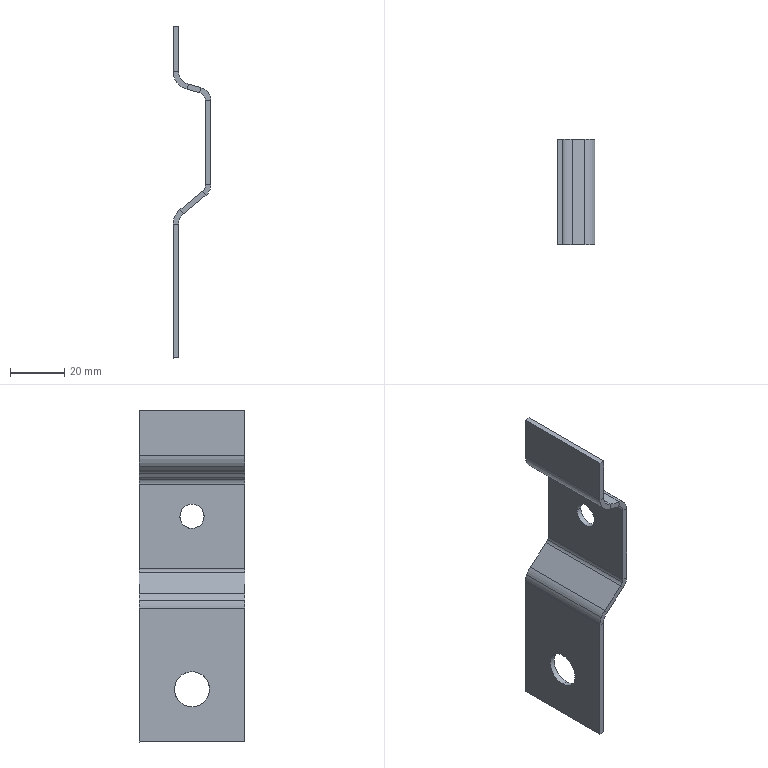Part | NX | features BREP 1 | 1 solid | 46 faces | box 14 x 39 x 122.887 mm | volume 10128 mm3 | plane 30 | cylinder 16 | commonest cylinder face diameters 6 x4 10 x4 14 x4 9 x2 13 x2
STEP:
#1=CARTESIAN_POINT('',(580.388,46.572,344.883));
#2=VERTEX_POINT('',#1);
#3=CARTESIAN_POINT('',(580.388,7.572,344.883));
#4=VERTEX_POINT('',#3);
#5=CARTESIAN_POINT('',(580.388,27.072,344.883));
#6=DIRECTION('',(0.,-1.,0.));
#7=VECTOR('',#6,1000.);
#8=LINE('',#5,#7);
#9=EDGE_CURVE('',#2,#4,#8,.T.);
#10=ORIENTED_EDGE('',*,*,#9,.F.);
#11=CARTESIAN_POINT('',(580.388,46.572,328.184));
#12=VERTEX_POINT('',#11);
#13=CARTESIAN_POINT('',(580.388,46.572,336.534));
#14=DIRECTION('',(0.,0.,1.));
#15=VECTOR('',#14,1000.);
#16=LINE('',#13,#15);
#17=EDGE_CURVE('',#12,#2,#16,.T.);
#18=ORIENTED_EDGE('',*,*,#17,.F.);
#19=CARTESIAN_POINT('',(580.388,7.572,328.184));
#20=VERTEX_POINT('',#19);
#21=CARTESIAN_POINT('',(580.388,27.072,328.184));
#22=DIRECTION('',(0.,1.,-0.000000573));
#23=VECTOR('',#22,1000.);
#24=LINE('',#21,#23);
#25=EDGE_CURVE('',#20,#12,#24,.T.);
#26=ORIENTED_EDGE('',*,*,#25,.F.);
#27=CARTESIAN_POINT('',(580.388,7.572,336.534));
#28=DIRECTION('',(0.,0.,1.));
#29=VECTOR('',#28,1000.);
#30=LINE('',#27,#29);
#31=EDGE_CURVE('',#20,#4,#30,.T.);
#32=ORIENTED_EDGE('',*,*,#31,.T.);
#33=EDGE_LOOP('',(#10,#18,#26,#32));
#34=FACE_BOUND('',#33,.T.);
#35=CARTESIAN_POINT('',(580.388,46.572,328.184));
#36=DIRECTION('',(-1.,0.,0.));
#37=DIRECTION('',(0.,-1.,0.));
#38=AXIS2_PLACEMENT_3D('',#35,#36,#37);
#39=PLANE('',#38);
#40=ADVANCED_FACE('',(#34),#39,.T.);
#41=CARTESIAN_POINT('',(582.388,46.572,344.883));
#42=VERTEX_POINT('',#41);
#43=CARTESIAN_POINT('',(581.388,46.572,344.883));
#44=DIRECTION('',(-1.,0.,0.));
#45=VECTOR('',#44,1000.);
#46=LINE('',#43,#45);
#47=EDGE_CURVE('',#42,#2,#46,.T.);
#48=ORIENTED_EDGE('',*,*,#47,.T.);
#49=ORIENTED_EDGE('',*,*,#9,.T.);
#50=CARTESIAN_POINT('',(582.388,7.572,344.883));
#51=VERTEX_POINT('',#50);
#52=CARTESIAN_POINT('',(581.388,7.572,344.883));
#53=DIRECTION('',(-1.,0.,0.));
#54=VECTOR('',#53,1000.);
#55=LINE('',#52,#54);
#56=EDGE_CURVE('',#51,#4,#55,.T.);
#57=ORIENTED_EDGE('',*,*,#56,.F.);
#58=CARTESIAN_POINT('',(582.388,27.072,344.883));
#59=DIRECTION('',(0.,-1.,0.));
#60=VECTOR('',#59,1000.);
#61=LINE('',#58,#60);
#62=EDGE_CURVE('',#42,#51,#61,.T.);
#63=ORIENTED_EDGE('',*,*,#62,.F.);
#64=EDGE_LOOP('',(#48,#49,#57,#63));
#65=FACE_BOUND('',#64,.T.);
#66=CARTESIAN_POINT('',(582.388,46.572,344.883));
#67=DIRECTION('',(0.,0.,-1.));
#68=DIRECTION('',(0.,-1.,0.));
#69=AXIS2_PLACEMENT_3D('',#66,#67,#68);
#70=PLANE('',#69);
#71=ADVANCED_FACE('',(#65),#70,.F.);
#72=CARTESIAN_POINT('',(582.388,46.572,328.184));
#73=VERTEX_POINT('',#72);
#74=CARTESIAN_POINT('',(582.388,46.572,336.534));
#75=DIRECTION('',(0.,0.,1.));
#76=VECTOR('',#75,1000.);
#77=LINE('',#74,#76);
#78=EDGE_CURVE('',#73,#42,#77,.T.);
#79=ORIENTED_EDGE('',*,*,#78,.F.);
#80=CARTESIAN_POINT('',(581.388,46.572,328.184));
#81=DIRECTION('',(-1.,0.,0.000000001));
#82=VECTOR('',#81,1000.);
#83=LINE('',#80,#82);
#84=EDGE_CURVE('',#73,#12,#83,.T.);
#85=ORIENTED_EDGE('',*,*,#84,.T.);
#86=ORIENTED_EDGE('',*,*,#17,.T.);
#87=ORIENTED_EDGE('',*,*,#47,.F.);
#88=EDGE_LOOP('',(#79,#85,#86,#87));
#89=FACE_BOUND('',#88,.T.);
#90=CARTESIAN_POINT('',(582.388,46.572,328.184));
#91=DIRECTION('',(0.,-1.,0.));
#92=DIRECTION('',(0.,0.,1.));
#93=AXIS2_PLACEMENT_3D('',#90,#91,#92);
#94=PLANE('',#93);
#95=ADVANCED_FACE('',(#89),#94,.F.);
#96=CARTESIAN_POINT('',(581.835,7.572,323.923));
#97=VERTEX_POINT('',#96);
#98=CARTESIAN_POINT('',(581.835,46.572,323.923));
#99=VERTEX_POINT('',#98);
#100=CARTESIAN_POINT('',(581.835,27.072,323.923));
#101=DIRECTION('',(0.,1.,-0.000000573));
#102=VECTOR('',#101,1000.);
#103=LINE('',#100,#102);
#104=EDGE_CURVE('',#97,#99,#103,.T.);
#105=ORIENTED_EDGE('',*,*,#104,.T.);
#106=CARTESIAN_POINT('',(585.577,46.572,321.423));
#107=VERTEX_POINT('',#106);
#108=CARTESIAN_POINT('',(587.388,46.572,328.184));
#109=DIRECTION('',(0.,1.,-0.000000573));
#110=DIRECTION('',(1.,0.,0.));
#111=AXIS2_PLACEMENT_3D('',#108,#109,#110);
#112=CIRCLE('',#111,7.);
#113=EDGE_CURVE('',#107,#99,#112,.T.);
#114=ORIENTED_EDGE('',*,*,#113,.F.);
#115=CARTESIAN_POINT('',(585.577,7.572,321.423));
#116=VERTEX_POINT('',#115);
#117=CARTESIAN_POINT('',(585.577,46.572,321.423));
#118=CARTESIAN_POINT('',(585.577,36.822,321.423));
#119=CARTESIAN_POINT('',(585.577,27.072,321.423));
#120=CARTESIAN_POINT('',(585.577,17.322,321.423));
#121=CARTESIAN_POINT('',(585.577,7.572,321.423));
#122=B_SPLINE_CURVE_WITH_KNOTS('',4,(#117,#118,#119,#120,#121),.UNSPECIFIED.,.F.,.F.,(5,5),(16.4,55.4),.UNSPECIFIED.);
#123=EDGE_CURVE('',#107,#116,#122,.T.);
#124=ORIENTED_EDGE('',*,*,#123,.T.);
#125=CARTESIAN_POINT('',(587.388,7.572,328.184));
#126=DIRECTION('',(0.,1.,-0.000000573));
#127=DIRECTION('',(1.,0.,0.));
#128=AXIS2_PLACEMENT_3D('',#125,#126,#127);
#129=CIRCLE('',#128,7.);
#130=EDGE_CURVE('',#116,#97,#129,.T.);
#131=ORIENTED_EDGE('',*,*,#130,.T.);
#132=EDGE_LOOP('',(#105,#114,#124,#131));
#133=FACE_BOUND('',#132,.T.);
#134=CARTESIAN_POINT('',(587.388,27.072,328.184));
#135=DIRECTION('',(0.,1.,-0.000000573));
#136=DIRECTION('',(0.7934,0.000000348,0.6088));
#137=AXIS2_PLACEMENT_3D('',#134,#135,#136);
#138=CYLINDRICAL_SURFACE('',#137,7.);
#139=ADVANCED_FACE('',(#133),#138,.T.);
#140=ORIENTED_EDGE('',*,*,#104,.F.);
#141=CARTESIAN_POINT('',(587.388,7.572,328.184));
#142=DIRECTION('',(0.,1.,-0.000000573));
#143=DIRECTION('',(1.,0.,0.));
#144=AXIS2_PLACEMENT_3D('',#141,#142,#143);
#145=CIRCLE('',#144,7.);
#146=EDGE_CURVE('',#97,#20,#145,.T.);
#147=ORIENTED_EDGE('',*,*,#146,.T.);
#148=ORIENTED_EDGE('',*,*,#25,.T.);
#149=CARTESIAN_POINT('',(587.388,46.572,328.184));
#150=DIRECTION('',(0.,1.,-0.000000573));
#151=DIRECTION('',(1.,0.,0.));
#152=AXIS2_PLACEMENT_3D('',#149,#150,#151);
#153=CIRCLE('',#152,7.);
#154=EDGE_CURVE('',#99,#12,#153,.T.);
#155=ORIENTED_EDGE('',*,*,#154,.F.);
#156=EDGE_LOOP('',(#140,#147,#148,#155));
#157=FACE_BOUND('',#156,.T.);
#158=CARTESIAN_POINT('',(587.388,27.072,328.184));
#159=DIRECTION('',(0.,1.,-0.000000573));
#160=DIRECTION('',(-0.7934,-0.000000348,-0.6088));
#161=AXIS2_PLACEMENT_3D('',#158,#159,#160);
#162=CYLINDRICAL_SURFACE('',#161,7.);
#163=ADVANCED_FACE('',(#157),#162,.T.);
#164=ORIENTED_EDGE('',*,*,#56,.T.);
#165=ORIENTED_EDGE('',*,*,#31,.F.);
#166=CARTESIAN_POINT('',(582.388,7.572,328.184));
#167=VERTEX_POINT('',#166);
#168=CARTESIAN_POINT('',(581.388,7.572,328.184));
#169=DIRECTION('',(-1.,0.,0.));
#170=VECTOR('',#169,1000.);
#171=LINE('',#168,#170);
#172=EDGE_CURVE('',#167,#20,#171,.T.);
#173=ORIENTED_EDGE('',*,*,#172,.F.);
#174=CARTESIAN_POINT('',(582.388,7.572,336.534));
#175=DIRECTION('',(0.,0.,1.));
#176=VECTOR('',#175,1000.);
#177=LINE('',#174,#176);
#178=EDGE_CURVE('',#167,#51,#177,.T.);
#179=ORIENTED_EDGE('',*,*,#178,.T.);
#180=EDGE_LOOP('',(#164,#165,#173,#179));
#181=FACE_BOUND('',#180,.T.);
#182=CARTESIAN_POINT('',(582.388,7.572,328.184));
#183=DIRECTION('',(0.,-1.,0.));
#184=DIRECTION('',(0.,0.,1.));
#185=AXIS2_PLACEMENT_3D('',#182,#183,#184);
#186=PLANE('',#185);
#187=ADVANCED_FACE('',(#181),#186,.T.);
#188=ORIENTED_EDGE('',*,*,#178,.F.);
#189=CARTESIAN_POINT('',(582.388,27.072,328.184));
#190=DIRECTION('',(0.,1.,-0.000000573));
#191=VECTOR('',#190,1000.);
#192=LINE('',#189,#191);
#193=EDGE_CURVE('',#167,#73,#192,.T.);
#194=ORIENTED_EDGE('',*,*,#193,.T.);
#195=ORIENTED_EDGE('',*,*,#78,.T.);
#196=ORIENTED_EDGE('',*,*,#62,.T.);
#197=EDGE_LOOP('',(#188,#194,#195,#196));
#198=FACE_BOUND('',#197,.T.);
#199=CARTESIAN_POINT('',(582.388,46.572,328.184));
#200=DIRECTION('',(-1.,0.,0.));
#201=DIRECTION('',(0.,-1.,0.));
#202=AXIS2_PLACEMENT_3D('',#199,#200,#201);
#203=PLANE('',#202);
#204=ADVANCED_FACE('',(#198),#203,.F.);
#205=CARTESIAN_POINT('',(586.094,46.572,323.355));
#206=VERTEX_POINT('',#205);
#207=CARTESIAN_POINT('',(587.388,46.572,328.184));
#208=DIRECTION('',(0.,1.,-0.000000573));
#209=DIRECTION('',(1.,0.,0.));
#210=AXIS2_PLACEMENT_3D('',#207,#208,#209);
#211=CIRCLE('',#210,5.);
#212=EDGE_CURVE('',#206,#73,#211,.T.);
#213=ORIENTED_EDGE('',*,*,#212,.F.);
#214=CARTESIAN_POINT('',(585.577,46.572,321.423));
#215=CARTESIAN_POINT('',(586.094,46.572,323.355));
#216=B_SPLINE_CURVE_WITH_KNOTS('',1,(#214,#215),.UNSPECIFIED.,.F.,.F.,(2,2),(-2.,0.),.UNSPECIFIED.);
#217=EDGE_CURVE('',#107,#206,#216,.T.);
#218=ORIENTED_EDGE('',*,*,#217,.F.);
#219=ORIENTED_EDGE('',*,*,#113,.T.);
#220=ORIENTED_EDGE('',*,*,#154,.T.);
#221=ORIENTED_EDGE('',*,*,#84,.F.);
#222=EDGE_LOOP('',(#213,#218,#219,#220,#221));
#223=FACE_BOUND('',#222,.T.);
#224=CARTESIAN_POINT('',(583.744,46.572,325.388));
#225=DIRECTION('',(0.,1.,-0.000000573));
#226=DIRECTION('',(0.7934,0.000000348,0.6088));
#227=AXIS2_PLACEMENT_3D('',#224,#225,#226);
#228=PLANE('',#227);
#229=ADVANCED_FACE('',(#223),#228,.T.);
#230=CARTESIAN_POINT('',(590.165,7.572,320.193));
#231=VERTEX_POINT('',#230);
#232=CARTESIAN_POINT('',(587.871,7.572,320.808));
#233=DIRECTION('',(0.9659,0.,-0.2588));
#234=VECTOR('',#233,1000.);
#235=LINE('',#232,#234);
#236=EDGE_CURVE('',#116,#231,#235,.T.);
#237=ORIENTED_EDGE('',*,*,#236,.F.);
#238=ORIENTED_EDGE('',*,*,#123,.F.);
#239=CARTESIAN_POINT('',(590.165,46.572,320.193));
#240=VERTEX_POINT('',#239);
#241=CARTESIAN_POINT('',(585.577,46.572,321.423));
#242=CARTESIAN_POINT('',(586.494,46.572,321.177));
#243=CARTESIAN_POINT('',(587.412,46.572,320.931));
#244=CARTESIAN_POINT('',(588.33,46.572,320.685));
#245=CARTESIAN_POINT('',(589.247,46.572,320.439));
#246=CARTESIAN_POINT('',(590.165,46.572,320.193));
#247=B_SPLINE_CURVE_WITH_KNOTS('',5,(#241,#242,#243,#244,#245,#246),.UNSPECIFIED.,.F.,.F.,(6,6),(0.,4.75),.UNSPECIFIED.);
#248=EDGE_CURVE('',#107,#240,#247,.T.);
#249=ORIENTED_EDGE('',*,*,#248,.T.);
#250=CARTESIAN_POINT('',(590.165,27.072,320.193));
#251=DIRECTION('',(0.,1.,-0.000000573));
#252=VECTOR('',#251,1000.);
#253=LINE('',#250,#252);
#254=EDGE_CURVE('',#231,#240,#253,.T.);
#255=ORIENTED_EDGE('',*,*,#254,.F.);
#256=EDGE_LOOP('',(#237,#238,#249,#255));
#257=FACE_BOUND('',#256,.T.);
#258=CARTESIAN_POINT('',(587.871,27.072,320.808));
#259=DIRECTION('',(0.2588,0.000000553,0.9659));
#260=DIRECTION('',(0.9659,0.,-0.2588));
#261=AXIS2_PLACEMENT_3D('',#258,#259,#260);
#262=PLANE('',#261);
#263=ADVANCED_FACE('',(#257),#262,.F.);
#264=ORIENTED_EDGE('',*,*,#172,.T.);
#265=ORIENTED_EDGE('',*,*,#146,.F.);
#266=ORIENTED_EDGE('',*,*,#130,.F.);
#267=CARTESIAN_POINT('',(586.094,7.572,323.355));
#268=VERTEX_POINT('',#267);
#269=CARTESIAN_POINT('',(585.835,7.572,322.389));
#270=DIRECTION('',(-0.2588,-0.000000553,-0.9659));
#271=VECTOR('',#270,1000.);
#272=LINE('',#269,#271);
#273=EDGE_CURVE('',#268,#116,#272,.T.);
#274=ORIENTED_EDGE('',*,*,#273,.F.);
#275=CARTESIAN_POINT('',(587.388,7.572,328.184));
#276=DIRECTION('',(0.,1.,-0.000000573));
#277=DIRECTION('',(1.,0.,0.));
#278=AXIS2_PLACEMENT_3D('',#275,#276,#277);
#279=CIRCLE('',#278,5.);
#280=EDGE_CURVE('',#268,#167,#279,.T.);
#281=ORIENTED_EDGE('',*,*,#280,.T.);
#282=EDGE_LOOP('',(#264,#265,#266,#274,#281));
#283=FACE_BOUND('',#282,.T.);
#284=CARTESIAN_POINT('',(583.744,7.572,325.388));
#285=DIRECTION('',(0.,1.,-0.000000573));
#286=DIRECTION('',(0.7934,0.000000348,0.6088));
#287=AXIS2_PLACEMENT_3D('',#284,#285,#286);
#288=PLANE('',#287);
#289=ADVANCED_FACE('',(#283),#288,.F.);
#290=ORIENTED_EDGE('',*,*,#280,.F.);
#291=CARTESIAN_POINT('',(586.094,46.572,323.355));
#292=CARTESIAN_POINT('',(586.094,40.472,323.355));
#293=CARTESIAN_POINT('',(586.094,34.372,323.355));
#294=CARTESIAN_POINT('',(586.094,28.272,323.355));
#295=CARTESIAN_POINT('',(586.094,20.472,323.355));
#296=CARTESIAN_POINT('',(586.094,12.672,323.355));
#297=CARTESIAN_POINT('',(586.094,10.972,323.355));
#298=CARTESIAN_POINT('',(586.094,9.272,323.355));
#299=CARTESIAN_POINT('',(586.094,7.572,323.355));
#300=B_SPLINE_CURVE_WITH_KNOTS('',5,(#291,#292,#293,#294,#295,#296,#297,#298,#299),.UNSPECIFIED.,.F.,.F.,(6,3,6),(16.4,46.9,55.4),.UNSPECIFIED.);
#301=EDGE_CURVE('',#206,#268,#300,.T.);
#302=ORIENTED_EDGE('',*,*,#301,.F.);
#303=ORIENTED_EDGE('',*,*,#212,.T.);
#304=ORIENTED_EDGE('',*,*,#193,.F.);
#305=EDGE_LOOP('',(#290,#302,#303,#304));
#306=FACE_BOUND('',#305,.T.);
#307=CARTESIAN_POINT('',(587.388,27.072,328.184));
#308=DIRECTION('',(0.,1.,-0.000000573));
#309=DIRECTION('',(-0.2588,-0.000000553,-0.9659));
#310=AXIS2_PLACEMENT_3D('',#307,#308,#309);
#311=CYLINDRICAL_SURFACE('',#310,5.);
#312=ADVANCED_FACE('',(#306),#311,.F.);
#313=CARTESIAN_POINT('',(590.683,46.572,322.125));
#314=VERTEX_POINT('',#313);
#315=CARTESIAN_POINT('',(590.424,46.572,321.159));
#316=DIRECTION('',(0.2588,0.000000553,0.9659));
#317=VECTOR('',#316,1000.);
#318=LINE('',#315,#317);
#319=EDGE_CURVE('',#240,#314,#318,.T.);
#320=ORIENTED_EDGE('',*,*,#319,.F.);
#321=ORIENTED_EDGE('',*,*,#248,.F.);
#322=ORIENTED_EDGE('',*,*,#217,.T.);
#323=CARTESIAN_POINT('',(586.094,46.572,323.355));
#324=CARTESIAN_POINT('',(587.012,46.572,323.109));
#325=CARTESIAN_POINT('',(587.93,46.572,322.863));
#326=CARTESIAN_POINT('',(588.847,46.572,322.617));
#327=CARTESIAN_POINT('',(589.765,46.572,322.371));
#328=CARTESIAN_POINT('',(590.683,46.572,322.125));
#329=B_SPLINE_CURVE_WITH_KNOTS('',5,(#323,#324,#325,#326,#327,#328),.UNSPECIFIED.,.F.,.F.,(6,6),(49.413,54.163),.UNSPECIFIED.);
#330=EDGE_CURVE('',#206,#314,#329,.T.);
#331=ORIENTED_EDGE('',*,*,#330,.T.);
#332=EDGE_LOOP('',(#320,#321,#322,#331));
#333=FACE_BOUND('',#332,.T.);
#334=CARTESIAN_POINT('',(588.13,46.572,321.774));
#335=DIRECTION('',(0.000000143,-1.,0.000000534));
#336=DIRECTION('',(0.,-0.000000534,-1.));
#337=AXIS2_PLACEMENT_3D('',#334,#335,#336);
#338=PLANE('',#337);
#339=ADVANCED_FACE('',(#333),#338,.F.);
#340=CARTESIAN_POINT('',(591.769,46.572,319.122));
#341=VERTEX_POINT('',#340);
#342=CARTESIAN_POINT('',(592.389,46.572,317.296));
#343=VERTEX_POINT('',#342);
#344=CARTESIAN_POINT('',(589.389,46.572,317.295));
#345=DIRECTION('',(0.,1.,-0.000000573));
#346=DIRECTION('',(1.,0.,0.));
#347=AXIS2_PLACEMENT_3D('',#344,#345,#346);
#348=CIRCLE('',#347,3.);
#349=EDGE_CURVE('',#341,#343,#348,.T.);
#350=ORIENTED_EDGE('',*,*,#349,.T.);
#351=CARTESIAN_POINT('',(592.389,7.572,317.296));
#352=VERTEX_POINT('',#351);
#353=CARTESIAN_POINT('',(592.389,27.072,317.296));
#354=DIRECTION('',(0.,1.,0.));
#355=VECTOR('',#354,1000.);
#356=LINE('',#353,#355);
#357=EDGE_CURVE('',#352,#343,#356,.T.);
#358=ORIENTED_EDGE('',*,*,#357,.F.);
#359=CARTESIAN_POINT('',(591.769,7.572,319.122));
#360=VERTEX_POINT('',#359);
#361=CARTESIAN_POINT('',(589.389,7.572,317.296));
#362=DIRECTION('',(0.,1.,-0.000000573));
#363=DIRECTION('',(1.,0.,0.));
#364=AXIS2_PLACEMENT_3D('',#361,#362,#363);
#365=CIRCLE('',#364,3.);
#366=EDGE_CURVE('',#360,#352,#365,.T.);
#367=ORIENTED_EDGE('',*,*,#366,.F.);
#368=CARTESIAN_POINT('',(591.769,27.072,319.122));
#369=DIRECTION('',(0.,1.,-0.000000573));
#370=VECTOR('',#369,1000.);
#371=LINE('',#368,#370);
#372=EDGE_CURVE('',#360,#341,#371,.T.);
#373=ORIENTED_EDGE('',*,*,#372,.T.);
#374=EDGE_LOOP('',(#350,#358,#367,#373));
#375=FACE_BOUND('',#374,.T.);
#376=CARTESIAN_POINT('',(589.389,27.072,317.295));
#377=DIRECTION('',(0.,1.,-0.000000573));
#378=DIRECTION('',(0.7934,0.000000348,0.6088));
#379=AXIS2_PLACEMENT_3D('',#376,#377,#378);
#380=CYLINDRICAL_SURFACE('',#379,3.);
#381=ADVANCED_FACE('',(#375),#380,.F.);
#382=CARTESIAN_POINT('',(589.389,7.572,317.296));
#383=DIRECTION('',(0.,1.,-0.000000573));
#384=DIRECTION('',(1.,0.,0.));
#385=AXIS2_PLACEMENT_3D('',#382,#383,#384);
#386=CIRCLE('',#385,3.);
#387=EDGE_CURVE('',#231,#360,#386,.T.);
#388=ORIENTED_EDGE('',*,*,#387,.F.);
#389=ORIENTED_EDGE('',*,*,#254,.T.);
#390=CARTESIAN_POINT('',(589.389,46.572,317.295));
#391=DIRECTION('',(0.,1.,-0.000000573));
#392=DIRECTION('',(1.,0.,0.));
#393=AXIS2_PLACEMENT_3D('',#390,#391,#392);
#394=CIRCLE('',#393,3.);
#395=EDGE_CURVE('',#240,#341,#394,.T.);
#396=ORIENTED_EDGE('',*,*,#395,.T.);
#397=ORIENTED_EDGE('',*,*,#372,.F.);
#398=EDGE_LOOP('',(#388,#389,#396,#397));
#399=FACE_BOUND('',#398,.T.);
#400=CARTESIAN_POINT('',(589.389,27.072,317.295));
#401=DIRECTION('',(0.,1.,-0.000000573));
#402=DIRECTION('',(-0.7934,-0.000000348,-0.6088));
#403=AXIS2_PLACEMENT_3D('',#400,#401,#402);
#404=CYLINDRICAL_SURFACE('',#403,3.);
#405=ADVANCED_FACE('',(#399),#404,.F.);
#406=CARTESIAN_POINT('',(590.683,7.572,322.125));
#407=VERTEX_POINT('',#406);
#408=CARTESIAN_POINT('',(586.094,7.572,323.355));
#409=CARTESIAN_POINT('',(587.012,7.572,323.109));
#410=CARTESIAN_POINT('',(587.93,7.572,322.863));
#411=CARTESIAN_POINT('',(588.847,7.572,322.617));
#412=CARTESIAN_POINT('',(589.765,7.572,322.371));
#413=CARTESIAN_POINT('',(590.683,7.572,322.125));
#414=B_SPLINE_CURVE_WITH_KNOTS('',5,(#408,#409,#410,#411,#412,#413),.UNSPECIFIED.,.F.,.F.,(6,6),(49.413,54.163),.UNSPECIFIED.);
#415=EDGE_CURVE('',#268,#407,#414,.T.);
#416=ORIENTED_EDGE('',*,*,#415,.F.);
#417=ORIENTED_EDGE('',*,*,#273,.T.);
#418=ORIENTED_EDGE('',*,*,#236,.T.);
#419=CARTESIAN_POINT('',(590.424,7.572,321.159));
#420=DIRECTION('',(0.2588,0.000000553,0.9659));
#421=VECTOR('',#420,1000.);
#422=LINE('',#419,#421);
#423=EDGE_CURVE('',#231,#407,#422,.T.);
#424=ORIENTED_EDGE('',*,*,#423,.T.);
#425=EDGE_LOOP('',(#416,#417,#418,#424));
#426=FACE_BOUND('',#425,.T.);
#427=CARTESIAN_POINT('',(586.094,7.572,323.355));
#428=DIRECTION('',(0.000000143,-1.,0.000000534));
#429=DIRECTION('',(0.9659,0.,-0.2588));
#430=AXIS2_PLACEMENT_3D('',#427,#428,#429);
#431=PLANE('',#430);
#432=ADVANCED_FACE('',(#426),#431,.T.);
#433=CARTESIAN_POINT('',(590.683,27.072,322.125));
#434=DIRECTION('',(0.,1.,-0.000000573));
#435=VECTOR('',#434,1000.);
#436=LINE('',#433,#435);
#437=EDGE_CURVE('',#407,#314,#436,.T.);
#438=ORIENTED_EDGE('',*,*,#437,.T.);
#439=ORIENTED_EDGE('',*,*,#330,.F.);
#440=ORIENTED_EDGE('',*,*,#301,.T.);
#441=ORIENTED_EDGE('',*,*,#415,.T.);
#442=EDGE_LOOP('',(#438,#439,#440,#441));
#443=FACE_BOUND('',#442,.T.);
#444=CARTESIAN_POINT('',(566.377,27.797,328.638));
#445=DIRECTION('',(0.2588,0.000000553,0.9659));
#446=DIRECTION('',(0.9659,0.,-0.2588));
#447=AXIS2_PLACEMENT_3D('',#444,#445,#446);
#448=PLANE('',#447);
#449=ADVANCED_FACE('',(#443),#448,.T.);
#450=CARTESIAN_POINT('',(594.389,46.572,317.295));
#451=VERTEX_POINT('',#450);
#452=CARTESIAN_POINT('',(593.389,46.572,317.295));
#453=DIRECTION('',(-1.,0.,0.));
#454=VECTOR('',#453,1000.);
#455=LINE('',#452,#454);
#456=EDGE_CURVE('',#451,#343,#455,.T.);
#457=ORIENTED_EDGE('',*,*,#456,.T.);
#458=ORIENTED_EDGE('',*,*,#349,.F.);
#459=ORIENTED_EDGE('',*,*,#395,.F.);
#460=ORIENTED_EDGE('',*,*,#319,.T.);
#461=CARTESIAN_POINT('',(589.389,46.572,317.295));
#462=DIRECTION('',(0.,1.,-0.000000573));
#463=DIRECTION('',(1.,0.,0.));
#464=AXIS2_PLACEMENT_3D('',#461,#462,#463);
#465=CIRCLE('',#464,5.);
#466=EDGE_CURVE('',#314,#451,#465,.T.);
#467=ORIENTED_EDGE('',*,*,#466,.T.);
#468=EDGE_LOOP('',(#457,#458,#459,#460,#467));
#469=FACE_BOUND('',#468,.T.);
#470=CARTESIAN_POINT('',(593.033,46.572,320.092));
#471=DIRECTION('',(0.,1.,-0.000000573));
#472=DIRECTION('',(0.7934,0.000000348,0.6088));
#473=AXIS2_PLACEMENT_3D('',#470,#471,#472);
#474=PLANE('',#473);
#475=ADVANCED_FACE('',(#469),#474,.T.);
#476=CARTESIAN_POINT('',(592.389,31.572,305.497));
#477=VERTEX_POINT('',#476);
#478=CARTESIAN_POINT('',(592.389,22.572,305.497));
#479=VERTEX_POINT('',#478);
#480=CARTESIAN_POINT('',(592.389,22.572,305.497));
#481=CARTESIAN_POINT('',(592.389,22.572,304.315));
#482=CARTESIAN_POINT('',(592.389,23.546,301.973));
#483=CARTESIAN_POINT('',(592.389,27.072,300.508));
#484=CARTESIAN_POINT('',(592.389,30.598,301.974));
#485=CARTESIAN_POINT('',(592.389,31.572,304.314));
#486=CARTESIAN_POINT('',(592.389,31.572,305.497));
#487=B_SPLINE_CURVE_WITH_KNOTS('',3,(#480,#481,#482,#483,#484,#485,#486),.UNSPECIFIED.,.F.,.F.,(4,1,1,1,4),(0.,0.25,0.5,0.75,1.),.UNSPECIFIED.);
#488=EDGE_CURVE('',#477,#479,#487,.F.);
#489=ORIENTED_EDGE('',*,*,#488,.F.);
#490=CARTESIAN_POINT('',(592.389,31.572,305.497));
#491=CARTESIAN_POINT('',(592.389,31.572,306.679));
#492=CARTESIAN_POINT('',(592.389,30.596,309.022));
#493=CARTESIAN_POINT('',(592.389,27.071,310.485));
#494=CARTESIAN_POINT('',(592.389,23.545,309.019));
#495=CARTESIAN_POINT('',(592.389,22.572,306.679));
#496=CARTESIAN_POINT('',(592.389,22.572,305.497));
#497=B_SPLINE_CURVE_WITH_KNOTS('',3,(#490,#491,#492,#493,#494,#495,#496),.UNSPECIFIED.,.F.,.F.,(4,1,1,1,4),(0.,0.25,0.5,0.75,1.),.UNSPECIFIED.);
#498=EDGE_CURVE('',#479,#477,#497,.F.);
#499=ORIENTED_EDGE('',*,*,#498,.F.);
#500=EDGE_LOOP('',(#489,#499));
#501=FACE_BOUND('',#500,.T.);
#502=CARTESIAN_POINT('',(592.389,7.572,286.103));
#503=VERTEX_POINT('',#502);
#504=CARTESIAN_POINT('',(592.389,46.572,286.103));
#505=VERTEX_POINT('',#504);
#506=CARTESIAN_POINT('',(592.389,27.072,286.103));
#507=DIRECTION('',(0.,1.,-0.000000573));
#508=VECTOR('',#507,1000.);
#509=LINE('',#506,#508);
#510=EDGE_CURVE('',#503,#505,#509,.T.);
#511=ORIENTED_EDGE('',*,*,#510,.F.);
#512=CARTESIAN_POINT('',(592.389,7.572,301.699));
#513=DIRECTION('',(0.,0.,-1.));
#514=VECTOR('',#513,1000.);
#515=LINE('',#512,#514);
#516=EDGE_CURVE('',#352,#503,#515,.T.);
#517=ORIENTED_EDGE('',*,*,#516,.F.);
#518=ORIENTED_EDGE('',*,*,#357,.T.);
#519=CARTESIAN_POINT('',(592.389,46.572,301.699));
#520=DIRECTION('',(0.,0.,1.));
#521=VECTOR('',#520,1000.);
#522=LINE('',#519,#521);
#523=EDGE_CURVE('',#505,#343,#522,.T.);
#524=ORIENTED_EDGE('',*,*,#523,.F.);
#525=EDGE_LOOP('',(#511,#517,#518,#524));
#526=FACE_BOUND('',#525,.T.);
#527=CARTESIAN_POINT('',(592.389,62.072,284.126));
#528=DIRECTION('',(-1.,0.,0.));
#529=DIRECTION('',(0.,0.,1.));
#530=AXIS2_PLACEMENT_3D('',#527,#528,#529);
#531=PLANE('',#530);
#532=ADVANCED_FACE('',(#501,#526),#531,.T.);
#533=CARTESIAN_POINT('',(594.389,7.572,317.296));
#534=VERTEX_POINT('',#533);
#535=CARTESIAN_POINT('',(589.389,7.572,317.296));
#536=DIRECTION('',(0.,1.,-0.000000573));
#537=DIRECTION('',(1.,0.,0.));
#538=AXIS2_PLACEMENT_3D('',#535,#536,#537);
#539=CIRCLE('',#538,5.);
#540=EDGE_CURVE('',#407,#534,#539,.T.);
#541=ORIENTED_EDGE('',*,*,#540,.F.);
#542=ORIENTED_EDGE('',*,*,#423,.F.);
#543=ORIENTED_EDGE('',*,*,#387,.T.);
#544=ORIENTED_EDGE('',*,*,#366,.T.);
#545=CARTESIAN_POINT('',(593.389,7.572,317.296));
#546=DIRECTION('',(-1.,0.,0.));
#547=VECTOR('',#546,1000.);
#548=LINE('',#545,#547);
#549=EDGE_CURVE('',#534,#352,#548,.T.);
#550=ORIENTED_EDGE('',*,*,#549,.F.);
#551=EDGE_LOOP('',(#541,#542,#543,#544,#550));
#552=FACE_BOUND('',#551,.T.);
#553=CARTESIAN_POINT('',(593.033,7.572,320.092));
#554=DIRECTION('',(0.,1.,-0.000000573));
#555=DIRECTION('',(0.7934,0.000000348,0.6088));
#556=AXIS2_PLACEMENT_3D('',#553,#554,#555);
#557=PLANE('',#556);
#558=ADVANCED_FACE('',(#552),#557,.F.);
#559=CARTESIAN_POINT('',(594.389,22.572,305.496));
#560=VERTEX_POINT('',#559);
#561=CARTESIAN_POINT('',(592.389,22.572,305.497));
#562=CARTESIAN_POINT('',(593.055,22.572,305.497));
#563=CARTESIAN_POINT('',(593.722,22.572,305.497));
#564=CARTESIAN_POINT('',(594.389,22.572,305.497));
#565=B_SPLINE_CURVE_WITH_KNOTS('',3,(#561,#562,#563,#564),.UNSPECIFIED.,.F.,.F.,(4,4),(0.,1.),.UNSPECIFIED.);
#566=EDGE_CURVE('',#560,#479,#565,.F.);
#567=ORIENTED_EDGE('',*,*,#566,.F.);
#568=CARTESIAN_POINT('',(594.389,31.572,305.497));
#569=VERTEX_POINT('',#568);
#570=CARTESIAN_POINT('',(594.389,31.572,305.497));
#571=CARTESIAN_POINT('',(594.389,31.572,304.304));
#572=CARTESIAN_POINT('',(594.389,30.597,301.98));
#573=CARTESIAN_POINT('',(594.389,27.073,300.505));
#574=CARTESIAN_POINT('',(594.389,23.546,301.979));
#575=CARTESIAN_POINT('',(594.389,22.572,304.302));
#576=CARTESIAN_POINT('',(594.389,22.572,305.496));
#577=B_SPLINE_CURVE_WITH_KNOTS('',3,(#570,#571,#572,#573,#574,#575,#576),.UNSPECIFIED.,.F.,.F.,(4,1,1,1,4),(0.,0.25,0.5,0.75,0.9999),.UNSPECIFIED.);
#578=EDGE_CURVE('',#569,#560,#577,.T.);
#579=ORIENTED_EDGE('',*,*,#578,.F.);
#580=CARTESIAN_POINT('',(594.389,31.572,305.497));
#581=CARTESIAN_POINT('',(593.722,31.572,305.497));
#582=CARTESIAN_POINT('',(593.055,31.572,305.497));
#583=CARTESIAN_POINT('',(592.389,31.572,305.497));
#584=B_SPLINE_CURVE_WITH_KNOTS('',3,(#580,#581,#582,#583),.UNSPECIFIED.,.F.,.F.,(4,4),(0.,1.),.UNSPECIFIED.);
#585=EDGE_CURVE('',#569,#477,#584,.T.);
#586=ORIENTED_EDGE('',*,*,#585,.T.);
#587=ORIENTED_EDGE('',*,*,#488,.T.);
#588=EDGE_LOOP('',(#567,#579,#586,#587));
#589=FACE_BOUND('',#588,.T.);
#590=CARTESIAN_POINT('',(594.389,27.072,305.497));
#591=DIRECTION('',(1.,0.,0.));
#592=DIRECTION('',(0.,0.,-1.));
#593=AXIS2_PLACEMENT_3D('',#590,#591,#592);
#594=CYLINDRICAL_SURFACE('',#593,4.5);
#595=ADVANCED_FACE('',(#589),#594,.F.);
#596=ORIENTED_EDGE('',*,*,#498,.T.);
#597=ORIENTED_EDGE('',*,*,#585,.F.);
#598=CARTESIAN_POINT('',(594.389,22.572,305.497));
#599=CARTESIAN_POINT('',(594.389,22.572,306.678));
#600=CARTESIAN_POINT('',(594.389,23.546,309.019));
#601=CARTESIAN_POINT('',(594.389,27.07,310.484));
#602=CARTESIAN_POINT('',(594.389,30.596,309.022));
#603=CARTESIAN_POINT('',(594.389,31.572,306.679));
#604=CARTESIAN_POINT('',(594.389,31.572,305.497));
#605=B_SPLINE_CURVE_WITH_KNOTS('',3,(#598,#599,#600,#601,#602,#603,#604),.UNSPECIFIED.,.F.,.F.,(4,1,1,1,4),(0.,0.25,0.5,0.75,0.9999),.UNSPECIFIED.);
#606=EDGE_CURVE('',#560,#569,#605,.T.);
#607=ORIENTED_EDGE('',*,*,#606,.F.);
#608=ORIENTED_EDGE('',*,*,#566,.T.);
#609=EDGE_LOOP('',(#596,#597,#607,#608));
#610=FACE_BOUND('',#609,.T.);
#611=CARTESIAN_POINT('',(594.389,27.072,305.497));
#612=DIRECTION('',(1.,0.,0.));
#613=DIRECTION('',(0.,0.,-1.));
#614=AXIS2_PLACEMENT_3D('',#611,#612,#613);
#615=CYLINDRICAL_SURFACE('',#614,4.5);
#616=ADVANCED_FACE('',(#610),#615,.F.);
#617=CARTESIAN_POINT('',(594.389,27.072,317.295));
#618=DIRECTION('',(0.,1.,-0.000000573));
#619=VECTOR('',#618,1000.);
#620=LINE('',#617,#619);
#621=EDGE_CURVE('',#534,#451,#620,.T.);
#622=ORIENTED_EDGE('',*,*,#621,.T.);
#623=ORIENTED_EDGE('',*,*,#466,.F.);
#624=ORIENTED_EDGE('',*,*,#437,.F.);
#625=ORIENTED_EDGE('',*,*,#540,.T.);
#626=EDGE_LOOP('',(#622,#623,#624,#625));
#627=FACE_BOUND('',#626,.T.);
#628=CARTESIAN_POINT('',(589.389,27.072,317.295));
#629=DIRECTION('',(0.,1.,-0.000000573));
#630=DIRECTION('',(0.2588,0.000000553,0.9659));
#631=AXIS2_PLACEMENT_3D('',#628,#629,#630);
#632=CYLINDRICAL_SURFACE('',#631,5.);
#633=ADVANCED_FACE('',(#627),#632,.T.);
#634=CARTESIAN_POINT('',(594.389,46.572,286.103));
#635=VERTEX_POINT('',#634);
#636=CARTESIAN_POINT('',(593.389,46.572,286.103));
#637=DIRECTION('',(1.,0.,0.));
#638=VECTOR('',#637,1000.);
#639=LINE('',#636,#638);
#640=EDGE_CURVE('',#505,#635,#639,.T.);
#641=ORIENTED_EDGE('',*,*,#640,.F.);
#642=ORIENTED_EDGE('',*,*,#523,.T.);
#643=ORIENTED_EDGE('',*,*,#456,.F.);
#644=CARTESIAN_POINT('',(594.389,46.572,301.699));
#645=DIRECTION('',(0.,0.000000051,-1.));
#646=VECTOR('',#645,1000.);
#647=LINE('',#644,#646);
#648=EDGE_CURVE('',#451,#635,#647,.T.);
#649=ORIENTED_EDGE('',*,*,#648,.T.);
#650=EDGE_LOOP('',(#641,#642,#643,#649));
#651=FACE_BOUND('',#650,.T.);
#652=CARTESIAN_POINT('',(594.389,46.572,301.699));
#653=DIRECTION('',(0.,1.,0.));
#654=DIRECTION('',(1.,0.,0.));
#655=AXIS2_PLACEMENT_3D('',#652,#653,#654);
#656=PLANE('',#655);
#657=ADVANCED_FACE('',(#651),#656,.T.);
#658=CARTESIAN_POINT('',(592.102,7.572,284.824));
#659=VERTEX_POINT('',#658);
#660=CARTESIAN_POINT('',(589.389,7.572,286.103));
#661=DIRECTION('',(0.,1.,-0.000000573));
#662=DIRECTION('',(1.,0.,0.));
#663=AXIS2_PLACEMENT_3D('',#660,#661,#662);
#664=CIRCLE('',#663,3.);
#665=EDGE_CURVE('',#503,#659,#664,.T.);
#666=ORIENTED_EDGE('',*,*,#665,.F.);
#667=ORIENTED_EDGE('',*,*,#510,.T.);
#668=CARTESIAN_POINT('',(592.102,46.572,284.824));
#669=VERTEX_POINT('',#668);
#670=CARTESIAN_POINT('',(589.389,46.572,286.103));
#671=DIRECTION('',(0.,1.,-0.000000573));
#672=DIRECTION('',(1.,0.,0.));
#673=AXIS2_PLACEMENT_3D('',#670,#671,#672);
#674=CIRCLE('',#673,3.);
#675=EDGE_CURVE('',#505,#669,#674,.T.);
#676=ORIENTED_EDGE('',*,*,#675,.T.);
#677=CARTESIAN_POINT('',(592.102,27.072,284.824));
#678=DIRECTION('',(0.,1.,-0.000000573));
#679=VECTOR('',#678,1000.);
#680=LINE('',#677,#679);
#681=EDGE_CURVE('',#659,#669,#680,.T.);
#682=ORIENTED_EDGE('',*,*,#681,.F.);
#683=EDGE_LOOP('',(#666,#667,#676,#682));
#684=FACE_BOUND('',#683,.T.);
#685=CARTESIAN_POINT('',(589.389,27.072,286.103));
#686=DIRECTION('',(0.,1.,-0.000000573));
#687=DIRECTION('',(-0.9045,0.000000244,0.4264));
#688=AXIS2_PLACEMENT_3D('',#685,#686,#687);
#689=CYLINDRICAL_SURFACE('',#688,3.);
#690=ADVANCED_FACE('',(#684),#689,.F.);
#691=CARTESIAN_POINT('',(594.389,7.572,286.103));
#692=VERTEX_POINT('',#691);
#693=CARTESIAN_POINT('',(594.389,7.572,301.699));
#694=DIRECTION('',(0.,0.000000051,-1.));
#695=VECTOR('',#694,1000.);
#696=LINE('',#693,#695);
#697=EDGE_CURVE('',#534,#692,#696,.T.);
#698=ORIENTED_EDGE('',*,*,#697,.F.);
#699=ORIENTED_EDGE('',*,*,#549,.T.);
#700=ORIENTED_EDGE('',*,*,#516,.T.);
#701=CARTESIAN_POINT('',(593.389,7.572,286.103));
#702=DIRECTION('',(1.,0.,0.));
#703=VECTOR('',#702,1000.);
#704=LINE('',#701,#703);
#705=EDGE_CURVE('',#503,#692,#704,.T.);
#706=ORIENTED_EDGE('',*,*,#705,.T.);
#707=EDGE_LOOP('',(#698,#699,#700,#706));
#708=FACE_BOUND('',#707,.T.);
#709=CARTESIAN_POINT('',(594.389,7.572,301.699));
#710=DIRECTION('',(0.,1.,0.));
#711=DIRECTION('',(1.,0.,0.));
#712=AXIS2_PLACEMENT_3D('',#709,#710,#711);
#713=PLANE('',#712);
#714=ADVANCED_FACE('',(#708),#713,.F.);
#715=CARTESIAN_POINT('',(591.298,46.572,283.789));
#716=VERTEX_POINT('',#715);
#717=CARTESIAN_POINT('',(589.389,46.572,286.103));
#718=DIRECTION('',(0.,1.,-0.000000573));
#719=DIRECTION('',(1.,0.,0.));
#720=AXIS2_PLACEMENT_3D('',#717,#718,#719);
#721=CIRCLE('',#720,3.);
#722=EDGE_CURVE('',#669,#716,#721,.T.);
#723=ORIENTED_EDGE('',*,*,#722,.T.);
#724=CARTESIAN_POINT('',(591.298,7.572,283.789));
#725=VERTEX_POINT('',#724);
#726=CARTESIAN_POINT('',(591.298,27.072,283.789));
#727=DIRECTION('',(0.,-1.,0.000000573));
#728=VECTOR('',#727,1000.);
#729=LINE('',#726,#728);
#730=EDGE_CURVE('',#716,#725,#729,.T.);
#731=ORIENTED_EDGE('',*,*,#730,.T.);
#732=CARTESIAN_POINT('',(589.389,7.572,286.103));
#733=DIRECTION('',(0.,1.,-0.000000573));
#734=DIRECTION('',(1.,0.,0.));
#735=AXIS2_PLACEMENT_3D('',#732,#733,#734);
#736=CIRCLE('',#735,3.);
#737=EDGE_CURVE('',#659,#725,#736,.T.);
#738=ORIENTED_EDGE('',*,*,#737,.F.);
#739=ORIENTED_EDGE('',*,*,#681,.T.);
#740=EDGE_LOOP('',(#723,#731,#738,#739));
#741=FACE_BOUND('',#740,.T.);
#742=CARTESIAN_POINT('',(589.389,27.072,286.103));
#743=DIRECTION('',(0.,1.,-0.000000573));
#744=DIRECTION('',(0.9045,-0.000000244,-0.4264));
#745=AXIS2_PLACEMENT_3D('',#742,#743,#744);
#746=CYLINDRICAL_SURFACE('',#745,3.);
#747=ADVANCED_FACE('',(#741),#746,.F.);
#748=ORIENTED_EDGE('',*,*,#606,.T.);
#749=ORIENTED_EDGE('',*,*,#578,.T.);
#750=EDGE_LOOP('',(#748,#749));
#751=FACE_BOUND('',#750,.T.);
#752=ORIENTED_EDGE('',*,*,#648,.F.);
#753=ORIENTED_EDGE('',*,*,#621,.F.);
#754=ORIENTED_EDGE('',*,*,#697,.T.);
#755=CARTESIAN_POINT('',(594.389,27.072,286.103));
#756=DIRECTION('',(0.,1.,-0.000000573));
#757=VECTOR('',#756,1000.);
#758=LINE('',#755,#757);
#759=EDGE_CURVE('',#692,#635,#758,.T.);
#760=ORIENTED_EDGE('',*,*,#759,.T.);
#761=EDGE_LOOP('',(#752,#753,#754,#760));
#762=FACE_BOUND('',#761,.T.);
#763=CARTESIAN_POINT('',(594.389,62.072,284.126));
#764=DIRECTION('',(-1.,0.,0.));
#765=DIRECTION('',(0.,0.,1.));
#766=AXIS2_PLACEMENT_3D('',#763,#764,#765);
#767=PLANE('',#766);
#768=ADVANCED_FACE('',(#751,#762),#767,.F.);
#769=CARTESIAN_POINT('',(592.571,46.572,282.247));
#770=VERTEX_POINT('',#769);
#771=CARTESIAN_POINT('',(591.934,46.572,283.018));
#772=DIRECTION('',(-0.6364,0.000000442,0.7714));
#773=VECTOR('',#772,1000.);
#774=LINE('',#771,#773);
#775=EDGE_CURVE('',#770,#716,#774,.T.);
#776=ORIENTED_EDGE('',*,*,#775,.T.);
#777=ORIENTED_EDGE('',*,*,#722,.F.);
#778=ORIENTED_EDGE('',*,*,#675,.F.);
#779=ORIENTED_EDGE('',*,*,#640,.T.);
#780=CARTESIAN_POINT('',(589.389,46.572,286.103));
#781=DIRECTION('',(0.,1.,-0.000000573));
#782=DIRECTION('',(1.,0.,0.));
#783=AXIS2_PLACEMENT_3D('',#780,#781,#782);
#784=CIRCLE('',#783,5.);
#785=EDGE_CURVE('',#635,#770,#784,.T.);
#786=ORIENTED_EDGE('',*,*,#785,.T.);
#787=EDGE_LOOP('',(#776,#777,#778,#779,#786));
#788=FACE_BOUND('',#787,.T.);
#789=CARTESIAN_POINT('',(593.743,46.572,284.051));
#790=DIRECTION('',(0.,1.,-0.000000573));
#791=DIRECTION('',(0.9045,-0.000000244,-0.4264));
#792=AXIS2_PLACEMENT_3D('',#789,#790,#791);
#793=PLANE('',#792);
#794=ADVANCED_FACE('',(#788),#793,.T.);
#795=CARTESIAN_POINT('',(592.571,7.572,282.247));
#796=VERTEX_POINT('',#795);
#797=CARTESIAN_POINT('',(589.389,7.572,286.103));
#798=DIRECTION('',(0.,1.,-0.000000573));
#799=DIRECTION('',(1.,0.,0.));
#800=AXIS2_PLACEMENT_3D('',#797,#798,#799);
#801=CIRCLE('',#800,5.);
#802=EDGE_CURVE('',#692,#796,#801,.T.);
#803=ORIENTED_EDGE('',*,*,#802,.F.);
#804=ORIENTED_EDGE('',*,*,#705,.F.);
#805=ORIENTED_EDGE('',*,*,#665,.T.);
#806=ORIENTED_EDGE('',*,*,#737,.T.);
#807=CARTESIAN_POINT('',(591.934,7.572,283.018));
#808=DIRECTION('',(-0.6364,0.000000442,0.7714));
#809=VECTOR('',#808,1000.);
#810=LINE('',#807,#809);
#811=EDGE_CURVE('',#796,#725,#810,.T.);
#812=ORIENTED_EDGE('',*,*,#811,.F.);
#813=EDGE_LOOP('',(#803,#804,#805,#806,#812));
#814=FACE_BOUND('',#813,.T.);
#815=CARTESIAN_POINT('',(593.743,7.572,284.051));
#816=DIRECTION('',(0.,1.,-0.000000573));
#817=DIRECTION('',(0.9045,-0.000000244,-0.4264));
#818=AXIS2_PLACEMENT_3D('',#815,#816,#817);
#819=PLANE('',#818);
#820=ADVANCED_FACE('',(#814),#819,.F.);
#821=CARTESIAN_POINT('',(582.934,7.572,276.889));
#822=VERTEX_POINT('',#821);
#823=CARTESIAN_POINT('',(582.934,46.572,276.889));
#824=VERTEX_POINT('',#823);
#825=CARTESIAN_POINT('',(582.934,27.072,276.889));
#826=DIRECTION('',(0.,1.,-0.000000573));
#827=VECTOR('',#826,1000.);
#828=LINE('',#825,#827);
#829=EDGE_CURVE('',#822,#824,#828,.T.);
#830=ORIENTED_EDGE('',*,*,#829,.F.);
#831=CARTESIAN_POINT('',(587.116,7.572,280.339));
#832=DIRECTION('',(-0.7714,0.,-0.6364));
#833=VECTOR('',#832,1000.);
#834=LINE('',#831,#833);
#835=EDGE_CURVE('',#725,#822,#834,.T.);
#836=ORIENTED_EDGE('',*,*,#835,.F.);
#837=ORIENTED_EDGE('',*,*,#730,.F.);
#838=CARTESIAN_POINT('',(587.116,46.572,280.339));
#839=DIRECTION('',(-0.7714,0.,-0.6364));
#840=VECTOR('',#839,1000.);
#841=LINE('',#838,#840);
#842=EDGE_CURVE('',#716,#824,#841,.T.);
#843=ORIENTED_EDGE('',*,*,#842,.T.);
#844=EDGE_LOOP('',(#830,#836,#837,#843));
#845=FACE_BOUND('',#844,.T.);
#846=CARTESIAN_POINT('',(593.116,27.072,285.289));
#847=DIRECTION('',(-0.6364,0.000000442,0.7714));
#848=DIRECTION('',(-0.7714,-0.000000364,-0.6364));
#849=AXIS2_PLACEMENT_3D('',#846,#847,#848);
#850=PLANE('',#849);
#851=ADVANCED_FACE('',(#845),#850,.T.);
#852=CARTESIAN_POINT('',(592.571,27.072,282.247));
#853=DIRECTION('',(0.,1.,-0.000000573));
#854=VECTOR('',#853,1000.);
#855=LINE('',#852,#854);
#856=EDGE_CURVE('',#796,#770,#855,.T.);
#857=ORIENTED_EDGE('',*,*,#856,.T.);
#858=ORIENTED_EDGE('',*,*,#785,.F.);
#859=ORIENTED_EDGE('',*,*,#759,.F.);
#860=ORIENTED_EDGE('',*,*,#802,.T.);
#861=EDGE_LOOP('',(#857,#858,#859,#860));
#862=FACE_BOUND('',#861,.T.);
#863=CARTESIAN_POINT('',(589.389,27.072,286.103));
#864=DIRECTION('',(0.,1.,-0.000000573));
#865=DIRECTION('',(1.,0.,0.));
#866=AXIS2_PLACEMENT_3D('',#863,#864,#865);
#867=CYLINDRICAL_SURFACE('',#866,5.);
#868=ADVANCED_FACE('',(#862),#867,.T.);
#869=CARTESIAN_POINT('',(584.207,46.572,275.346));
#870=VERTEX_POINT('',#869);
#871=CARTESIAN_POINT('',(583.57,46.572,276.118));
#872=DIRECTION('',(-0.6364,0.000000442,0.7714));
#873=VECTOR('',#872,1000.);
#874=LINE('',#871,#873);
#875=EDGE_CURVE('',#870,#824,#874,.T.);
#876=ORIENTED_EDGE('',*,*,#875,.T.);
#877=ORIENTED_EDGE('',*,*,#842,.F.);
#878=ORIENTED_EDGE('',*,*,#775,.F.);
#879=CARTESIAN_POINT('',(588.389,46.572,278.796));
#880=DIRECTION('',(-0.7714,-0.000000269,-0.6364));
#881=VECTOR('',#880,1000.);
#882=LINE('',#879,#881);
#883=EDGE_CURVE('',#770,#870,#882,.T.);
#884=ORIENTED_EDGE('',*,*,#883,.T.);
#885=EDGE_LOOP('',(#876,#877,#878,#884));
#886=FACE_BOUND('',#885,.T.);
#887=CARTESIAN_POINT('',(588.389,46.572,278.796));
#888=DIRECTION('',(-0.000000281,-1.,0.000000341));
#889=DIRECTION('',(1.,-0.000000281,0.));
#890=AXIS2_PLACEMENT_3D('',#887,#888,#889);
#891=PLANE('',#890);
#892=ADVANCED_FACE('',(#886),#891,.F.);
#893=CARTESIAN_POINT('',(584.207,7.572,275.346));
#894=VERTEX_POINT('',#893);
#895=CARTESIAN_POINT('',(588.389,7.572,278.796));
#896=DIRECTION('',(-0.7714,-0.000000269,-0.6364));
#897=VECTOR('',#896,1000.);
#898=LINE('',#895,#897);
#899=EDGE_CURVE('',#796,#894,#898,.T.);
#900=ORIENTED_EDGE('',*,*,#899,.F.);
#901=ORIENTED_EDGE('',*,*,#811,.T.);
#902=ORIENTED_EDGE('',*,*,#835,.T.);
#903=CARTESIAN_POINT('',(583.57,7.572,276.118));
#904=DIRECTION('',(-0.6364,0.000000442,0.7714));
#905=VECTOR('',#904,1000.);
#906=LINE('',#903,#905);
#907=EDGE_CURVE('',#894,#822,#906,.T.);
#908=ORIENTED_EDGE('',*,*,#907,.F.);
#909=EDGE_LOOP('',(#900,#901,#902,#908));
#910=FACE_BOUND('',#909,.T.);
#911=CARTESIAN_POINT('',(588.389,7.572,278.796));
#912=DIRECTION('',(-0.000000281,-1.,0.000000341));
#913=DIRECTION('',(1.,-0.000000281,0.));
#914=AXIS2_PLACEMENT_3D('',#911,#912,#913);
#915=PLANE('',#914);
#916=ADVANCED_FACE('',(#910),#915,.T.);
#917=CARTESIAN_POINT('',(581.057,7.572,274.474));
#918=VERTEX_POINT('',#917);
#919=CARTESIAN_POINT('',(581.057,46.572,274.474));
#920=VERTEX_POINT('',#919);
#921=CARTESIAN_POINT('',(581.057,27.072,274.474));
#922=DIRECTION('',(0.,1.,-0.000000573));
#923=VECTOR('',#922,1000.);
#924=LINE('',#921,#923);
#925=EDGE_CURVE('',#918,#920,#924,.T.);
#926=ORIENTED_EDGE('',*,*,#925,.F.);
#927=CARTESIAN_POINT('',(587.389,7.572,271.489));
#928=DIRECTION('',(0.,1.,-0.000000573));
#929=DIRECTION('',(1.,0.,0.));
#930=AXIS2_PLACEMENT_3D('',#927,#928,#929);
#931=CIRCLE('',#930,7.);
#932=EDGE_CURVE('',#918,#822,#931,.T.);
#933=ORIENTED_EDGE('',*,*,#932,.T.);
#934=ORIENTED_EDGE('',*,*,#829,.T.);
#935=CARTESIAN_POINT('',(587.389,46.572,271.489));
#936=DIRECTION('',(0.,1.,-0.000000573));
#937=DIRECTION('',(1.,0.,0.));
#938=AXIS2_PLACEMENT_3D('',#935,#936,#937);
#939=CIRCLE('',#938,7.);
#940=EDGE_CURVE('',#920,#824,#939,.T.);
#941=ORIENTED_EDGE('',*,*,#940,.F.);
#942=EDGE_LOOP('',(#926,#933,#934,#941));
#943=FACE_BOUND('',#942,.T.);
#944=CARTESIAN_POINT('',(587.389,27.072,271.489));
#945=DIRECTION('',(0.,1.,-0.000000573));
#946=DIRECTION('',(-0.9045,0.000000244,0.4264));
#947=AXIS2_PLACEMENT_3D('',#944,#945,#946);
#948=CYLINDRICAL_SURFACE('',#947,7.);
#949=ADVANCED_FACE('',(#943),#948,.T.);
#950=ORIENTED_EDGE('',*,*,#883,.F.);
#951=ORIENTED_EDGE('',*,*,#856,.F.);
#952=ORIENTED_EDGE('',*,*,#899,.T.);
#953=CARTESIAN_POINT('',(584.207,27.072,275.346));
#954=DIRECTION('',(0.,1.,-0.000000573));
#955=VECTOR('',#954,1000.);
#956=LINE('',#953,#955);
#957=EDGE_CURVE('',#894,#870,#956,.T.);
#958=ORIENTED_EDGE('',*,*,#957,.T.);
#959=EDGE_LOOP('',(#950,#951,#952,#958));
#960=FACE_BOUND('',#959,.T.);
#961=CARTESIAN_POINT('',(594.389,27.072,283.747));
#962=DIRECTION('',(-0.6364,0.000000442,0.7714));
#963=DIRECTION('',(-0.7714,-0.000000364,-0.6364));
#964=AXIS2_PLACEMENT_3D('',#961,#962,#963);
#965=PLANE('',#964);
#966=ADVANCED_FACE('',(#960),#965,.F.);
#967=CARTESIAN_POINT('',(580.389,46.572,271.489));
#968=VERTEX_POINT('',#967);
#969=CARTESIAN_POINT('',(582.389,46.572,271.489));
#970=VERTEX_POINT('',#969);
#971=CARTESIAN_POINT('',(581.389,46.572,271.489));
#972=DIRECTION('',(1.,0.,0.));
#973=VECTOR('',#972,1000.);
#974=LINE('',#971,#973);
#975=EDGE_CURVE('',#968,#970,#974,.T.);
#976=ORIENTED_EDGE('',*,*,#975,.F.);
#977=CARTESIAN_POINT('',(580.389,46.572,271.489));
#978=CARTESIAN_POINT('',(580.389,46.572,272.517));
#979=CARTESIAN_POINT('',(580.618,46.572,273.544));
#980=CARTESIAN_POINT('',(581.057,46.572,274.474));
#981=B_SPLINE_CURVE_WITH_KNOTS('',3,(#977,#978,#979,#980),.UNSPECIFIED.,.F.,.F.,(4,4),(0.,1.),.UNSPECIFIED.);
#982=EDGE_CURVE('',#968,#920,#981,.T.);
#983=ORIENTED_EDGE('',*,*,#982,.T.);
#984=ORIENTED_EDGE('',*,*,#940,.T.);
#985=ORIENTED_EDGE('',*,*,#875,.F.);
#986=CARTESIAN_POINT('',(587.389,46.572,271.489));
#987=DIRECTION('',(0.,1.,-0.000000573));
#988=DIRECTION('',(1.,0.,0.));
#989=AXIS2_PLACEMENT_3D('',#986,#987,#988);
#990=CIRCLE('',#989,5.);
#991=EDGE_CURVE('',#970,#870,#990,.T.);
#992=ORIENTED_EDGE('',*,*,#991,.F.);
#993=EDGE_LOOP('',(#976,#983,#984,#985,#992));
#994=FACE_BOUND('',#993,.T.);
#995=CARTESIAN_POINT('',(583.035,46.572,273.542));
#996=DIRECTION('',(0.,1.,-0.000000573));
#997=DIRECTION('',(0.9045,-0.000000244,-0.4264));
#998=AXIS2_PLACEMENT_3D('',#995,#996,#997);
#999=PLANE('',#998);
#1000=ADVANCED_FACE('',(#994),#999,.T.);
#1001=CARTESIAN_POINT('',(582.389,7.572,271.489));
#1002=VERTEX_POINT('',#1001);
#1003=CARTESIAN_POINT('',(587.389,7.572,271.489));
#1004=DIRECTION('',(0.,1.,-0.000000573));
#1005=DIRECTION('',(1.,0.,0.));
#1006=AXIS2_PLACEMENT_3D('',#1003,#1004,#1005);
#1007=CIRCLE('',#1006,5.);
#1008=EDGE_CURVE('',#1002,#894,#1007,.T.);
#1009=ORIENTED_EDGE('',*,*,#1008,.T.);
#1010=ORIENTED_EDGE('',*,*,#907,.T.);
#1011=ORIENTED_EDGE('',*,*,#932,.F.);
#1012=CARTESIAN_POINT('',(580.389,7.572,271.489));
#1013=VERTEX_POINT('',#1012);
#1014=CARTESIAN_POINT('',(581.057,7.572,274.474));
#1015=CARTESIAN_POINT('',(580.619,7.572,273.545));
#1016=CARTESIAN_POINT('',(580.389,7.572,272.518));
#1017=CARTESIAN_POINT('',(580.389,7.572,271.489));
#1018=B_SPLINE_CURVE_WITH_KNOTS('',3,(#1014,#1015,#1016,#1017),.UNSPECIFIED.,.F.,.F.,(4,4),(0.,1.),.UNSPECIFIED.);
#1019=EDGE_CURVE('',#1013,#918,#1018,.F.);
#1020=ORIENTED_EDGE('',*,*,#1019,.F.);
#1021=CARTESIAN_POINT('',(581.389,7.572,271.489));
#1022=DIRECTION('',(1.,0.,0.));
#1023=VECTOR('',#1022,1000.);
#1024=LINE('',#1021,#1023);
#1025=EDGE_CURVE('',#1013,#1002,#1024,.T.);
#1026=ORIENTED_EDGE('',*,*,#1025,.T.);
#1027=EDGE_LOOP('',(#1009,#1010,#1011,#1020,#1026));
#1028=FACE_BOUND('',#1027,.T.);
#1029=CARTESIAN_POINT('',(583.035,7.572,273.542));
#1030=DIRECTION('',(0.,1.,-0.000000573));
#1031=DIRECTION('',(0.9045,-0.000000244,-0.4264));
#1032=AXIS2_PLACEMENT_3D('',#1029,#1030,#1031);
#1033=PLANE('',#1032);
#1034=ADVANCED_FACE('',(#1028),#1033,.F.);
#1035=ORIENTED_EDGE('',*,*,#925,.T.);
#1036=ORIENTED_EDGE('',*,*,#982,.F.);
#1037=CARTESIAN_POINT('',(580.389,27.072,271.489));
#1038=DIRECTION('',(0.,-1.,0.000000573));
#1039=VECTOR('',#1038,1000.);
#1040=LINE('',#1037,#1039);
#1041=EDGE_CURVE('',#968,#1013,#1040,.T.);
#1042=ORIENTED_EDGE('',*,*,#1041,.T.);
#1043=ORIENTED_EDGE('',*,*,#1019,.T.);
#1044=EDGE_LOOP('',(#1035,#1036,#1042,#1043));
#1045=FACE_BOUND('',#1044,.T.);
#1046=CARTESIAN_POINT('',(587.389,27.072,271.489));
#1047=DIRECTION('',(0.,1.,-0.000000573));
#1048=DIRECTION('',(0.9045,-0.000000244,-0.4264));
#1049=AXIS2_PLACEMENT_3D('',#1046,#1047,#1048);
#1050=CYLINDRICAL_SURFACE('',#1049,7.);
#1051=ADVANCED_FACE('',(#1045),#1050,.T.);
#1052=ORIENTED_EDGE('',*,*,#991,.T.);
#1053=ORIENTED_EDGE('',*,*,#957,.F.);
#1054=ORIENTED_EDGE('',*,*,#1008,.F.);
#1055=CARTESIAN_POINT('',(582.389,27.072,271.489));
#1056=DIRECTION('',(0.,1.,-0.000000573));
#1057=VECTOR('',#1056,1000.);
#1058=LINE('',#1055,#1057);
#1059=EDGE_CURVE('',#1002,#970,#1058,.T.);
#1060=ORIENTED_EDGE('',*,*,#1059,.T.);
#1061=EDGE_LOOP('',(#1052,#1053,#1054,#1060));
#1062=FACE_BOUND('',#1061,.T.);
#1063=CARTESIAN_POINT('',(587.389,27.072,271.489));
#1064=DIRECTION('',(0.,1.,-0.000000573));
#1065=DIRECTION('',(-1.,0.,0.));
#1066=AXIS2_PLACEMENT_3D('',#1063,#1064,#1065);
#1067=CYLINDRICAL_SURFACE('',#1066,5.);
#1068=ADVANCED_FACE('',(#1062),#1067,.F.);
#1069=CARTESIAN_POINT('',(580.389,46.572,221.997));
#1070=VERTEX_POINT('',#1069);
#1071=CARTESIAN_POINT('',(582.389,46.572,221.997));
#1072=VERTEX_POINT('',#1071);
#1073=CARTESIAN_POINT('',(581.389,46.572,221.997));
#1074=DIRECTION('',(1.,0.,0.));
#1075=VECTOR('',#1074,1000.);
#1076=LINE('',#1073,#1075);
#1077=EDGE_CURVE('',#1070,#1072,#1076,.T.);
#1078=ORIENTED_EDGE('',*,*,#1077,.F.);
#1079=CARTESIAN_POINT('',(580.389,46.572,221.997));
#1080=CARTESIAN_POINT('',(580.389,46.572,238.494));
#1081=CARTESIAN_POINT('',(580.389,46.572,254.992));
#1082=CARTESIAN_POINT('',(580.389,46.572,271.489));
#1083=B_SPLINE_CURVE_WITH_KNOTS('',3,(#1079,#1080,#1081,#1082),.UNSPECIFIED.,.F.,.F.,(4,4),(0.,1.),.UNSPECIFIED.);
#1084=EDGE_CURVE('',#968,#1070,#1083,.F.);
#1085=ORIENTED_EDGE('',*,*,#1084,.F.);
#1086=ORIENTED_EDGE('',*,*,#975,.T.);
#1087=CARTESIAN_POINT('',(582.389,46.572,246.743));
#1088=DIRECTION('',(0.,0.000000024,-1.));
#1089=VECTOR('',#1088,1000.);
#1090=LINE('',#1087,#1089);
#1091=EDGE_CURVE('',#970,#1072,#1090,.T.);
#1092=ORIENTED_EDGE('',*,*,#1091,.T.);
#1093=EDGE_LOOP('',(#1078,#1085,#1086,#1092));
#1094=FACE_BOUND('',#1093,.T.);
#1095=CARTESIAN_POINT('',(582.389,46.572,246.743));
#1096=DIRECTION('',(0.,1.,0.));
#1097=DIRECTION('',(1.,0.,0.));
#1098=AXIS2_PLACEMENT_3D('',#1095,#1096,#1097);
#1099=PLANE('',#1098);
#1100=ADVANCED_FACE('',(#1094),#1099,.T.);
#1101=CARTESIAN_POINT('',(582.389,7.572,221.997));
#1102=VERTEX_POINT('',#1101);
#1103=CARTESIAN_POINT('',(582.389,27.072,221.997));
#1104=DIRECTION('',(0.,1.,0.));
#1105=VECTOR('',#1104,1000.);
#1106=LINE('',#1103,#1105);
#1107=EDGE_CURVE('',#1102,#1072,#1106,.T.);
#1108=ORIENTED_EDGE('',*,*,#1107,.F.);
#1109=CARTESIAN_POINT('',(580.389,7.572,221.997));
#1110=VERTEX_POINT('',#1109);
#1111=CARTESIAN_POINT('',(581.389,7.572,221.997));
#1112=DIRECTION('',(1.,0.,0.));
#1113=VECTOR('',#1112,1000.);
#1114=LINE('',#1111,#1113);
#1115=EDGE_CURVE('',#1110,#1102,#1114,.T.);
#1116=ORIENTED_EDGE('',*,*,#1115,.F.);
#1117=CARTESIAN_POINT('',(580.389,7.572,221.997));
#1118=CARTESIAN_POINT('',(580.389,20.572,221.997));
#1119=CARTESIAN_POINT('',(580.389,33.572,221.997));
#1120=CARTESIAN_POINT('',(580.389,46.572,221.997));
#1121=B_SPLINE_CURVE_WITH_KNOTS('',3,(#1117,#1118,#1119,#1120),.UNSPECIFIED.,.F.,.F.,(4,4),(0.,1.),.UNSPECIFIED.);
#1122=EDGE_CURVE('',#1110,#1070,#1121,.T.);
#1123=ORIENTED_EDGE('',*,*,#1122,.T.);
#1124=ORIENTED_EDGE('',*,*,#1077,.T.);
#1125=EDGE_LOOP('',(#1108,#1116,#1123,#1124));
#1126=FACE_BOUND('',#1125,.T.);
#1127=CARTESIAN_POINT('',(582.389,27.072,221.997));
#1128=DIRECTION('',(0.,0.,1.));
#1129=DIRECTION('',(1.,0.,0.));
#1130=AXIS2_PLACEMENT_3D('',#1127,#1128,#1129);
#1131=PLANE('',#1130);
#1132=ADVANCED_FACE('',(#1126),#1131,.F.);
#1133=CARTESIAN_POINT('',(582.389,7.572,246.743));
#1134=DIRECTION('',(0.,0.000000024,-1.));
#1135=VECTOR('',#1134,1000.);
#1136=LINE('',#1133,#1135);
#1137=EDGE_CURVE('',#1002,#1102,#1136,.T.);
#1138=ORIENTED_EDGE('',*,*,#1137,.F.);
#1139=ORIENTED_EDGE('',*,*,#1025,.F.);
#1140=CARTESIAN_POINT('',(580.389,7.572,271.489));
#1141=CARTESIAN_POINT('',(580.389,7.572,254.992));
#1142=CARTESIAN_POINT('',(580.389,7.572,238.494));
#1143=CARTESIAN_POINT('',(580.389,7.572,221.997));
#1144=B_SPLINE_CURVE_WITH_KNOTS('',3,(#1140,#1141,#1142,#1143),.UNSPECIFIED.,.F.,.F.,(4,4),(0.,1.),.UNSPECIFIED.);
#1145=EDGE_CURVE('',#1013,#1110,#1144,.T.);
#1146=ORIENTED_EDGE('',*,*,#1145,.T.);
#1147=ORIENTED_EDGE('',*,*,#1115,.T.);
#1148=EDGE_LOOP('',(#1138,#1139,#1146,#1147));
#1149=FACE_BOUND('',#1148,.T.);
#1150=CARTESIAN_POINT('',(582.389,7.572,246.743));
#1151=DIRECTION('',(0.,1.,0.));
#1152=DIRECTION('',(1.,0.,0.));
#1153=AXIS2_PLACEMENT_3D('',#1150,#1151,#1152);
#1154=PLANE('',#1153);
#1155=ADVANCED_FACE('',(#1149),#1154,.F.);
#1156=CARTESIAN_POINT('',(580.389,27.072,234.997));
#1157=VERTEX_POINT('',#1156);
#1158=CARTESIAN_POINT('',(580.389,27.072,247.997));
#1159=VERTEX_POINT('',#1158);
#1160=CARTESIAN_POINT('',(580.389,27.072,247.997));
#1161=CARTESIAN_POINT('',(580.389,25.347,247.996));
#1162=CARTESIAN_POINT('',(580.389,21.989,246.587));
#1163=CARTESIAN_POINT('',(580.389,19.863,241.494));
#1164=CARTESIAN_POINT('',(580.389,21.994,236.404));
#1165=CARTESIAN_POINT('',(580.389,25.348,234.997));
#1166=CARTESIAN_POINT('',(580.389,27.072,234.997));
#1167=B_SPLINE_CURVE_WITH_KNOTS('',3,(#1160,#1161,#1162,#1163,#1164,#1165,#1166),.UNSPECIFIED.,.F.,.F.,(4,1,1,1,4),(0.,0.25,0.5,0.75,1.),.UNSPECIFIED.);
#1168=EDGE_CURVE('',#1157,#1159,#1167,.F.);
#1169=ORIENTED_EDGE('',*,*,#1168,.F.);
#1170=CARTESIAN_POINT('',(580.389,27.072,234.997));
#1171=CARTESIAN_POINT('',(580.389,28.798,234.997));
#1172=CARTESIAN_POINT('',(580.389,32.156,236.406));
#1173=CARTESIAN_POINT('',(580.389,34.282,241.499));
#1174=CARTESIAN_POINT('',(580.389,32.15,246.589));
#1175=CARTESIAN_POINT('',(580.389,28.796,247.997));
#1176=CARTESIAN_POINT('',(580.389,27.072,247.997));
#1177=B_SPLINE_CURVE_WITH_KNOTS('',3,(#1170,#1171,#1172,#1173,#1174,#1175,#1176),.UNSPECIFIED.,.F.,.F.,(4,1,1,1,4),(0.,0.25,0.5,0.75,1.),.UNSPECIFIED.);
#1178=EDGE_CURVE('',#1159,#1157,#1177,.F.);
#1179=ORIENTED_EDGE('',*,*,#1178,.F.);
#1180=EDGE_LOOP('',(#1169,#1179));
#1181=FACE_BOUND('',#1180,.T.);
#1182=ORIENTED_EDGE('',*,*,#1041,.F.);
#1183=ORIENTED_EDGE('',*,*,#1084,.T.);
#1184=ORIENTED_EDGE('',*,*,#1122,.F.);
#1185=ORIENTED_EDGE('',*,*,#1145,.F.);
#1186=EDGE_LOOP('',(#1182,#1183,#1184,#1185));
#1187=FACE_BOUND('',#1186,.T.);
#1188=CARTESIAN_POINT('',(580.389,27.072,168.959));
#1189=DIRECTION('',(1.,0.,0.));
#1190=DIRECTION('',(0.,0.000000573,1.));
#1191=AXIS2_PLACEMENT_3D('',#1188,#1189,#1190);
#1192=PLANE('',#1191);
#1193=ADVANCED_FACE('',(#1181,#1187),#1192,.F.);
#1194=CARTESIAN_POINT('',(582.389,27.072,234.997));
#1195=VERTEX_POINT('',#1194);
#1196=CARTESIAN_POINT('',(582.389,27.072,247.997));
#1197=VERTEX_POINT('',#1196);
#1198=CARTESIAN_POINT('',(582.389,27.072,234.997));
#1199=CARTESIAN_POINT('',(582.389,25.349,234.997));
#1200=CARTESIAN_POINT('',(582.389,21.994,236.404));
#1201=CARTESIAN_POINT('',(582.389,19.863,241.494));
#1202=CARTESIAN_POINT('',(582.389,21.989,246.587));
#1203=CARTESIAN_POINT('',(582.389,25.346,247.996));
#1204=CARTESIAN_POINT('',(582.389,27.072,247.997));
#1205=B_SPLINE_CURVE_WITH_KNOTS('',3,(#1198,#1199,#1200,#1201,#1202,#1203,#1204),.UNSPECIFIED.,.F.,.F.,(4,1,1,1,4),(0.,0.25,0.5,0.75,1.),.UNSPECIFIED.);
#1206=EDGE_CURVE('',#1195,#1197,#1205,.T.);
#1207=ORIENTED_EDGE('',*,*,#1206,.T.);
#1208=CARTESIAN_POINT('',(582.389,27.072,247.997));
#1209=CARTESIAN_POINT('',(582.389,28.795,247.997));
#1210=CARTESIAN_POINT('',(582.389,32.151,246.589));
#1211=CARTESIAN_POINT('',(582.389,34.282,241.499));
#1212=CARTESIAN_POINT('',(582.389,32.155,236.406));
#1213=CARTESIAN_POINT('',(582.389,28.798,234.997));
#1214=CARTESIAN_POINT('',(582.389,27.072,234.997));
#1215=B_SPLINE_CURVE_WITH_KNOTS('',3,(#1208,#1209,#1210,#1211,#1212,#1213,#1214),.UNSPECIFIED.,.F.,.F.,(4,1,1,1,4),(0.,0.25,0.5,0.75,1.),.UNSPECIFIED.);
#1216=EDGE_CURVE('',#1197,#1195,#1215,.T.);
#1217=ORIENTED_EDGE('',*,*,#1216,.T.);
#1218=EDGE_LOOP('',(#1207,#1217));
#1219=FACE_BOUND('',#1218,.T.);
#1220=ORIENTED_EDGE('',*,*,#1137,.T.);
#1221=ORIENTED_EDGE('',*,*,#1107,.T.);
#1222=ORIENTED_EDGE('',*,*,#1091,.F.);
#1223=ORIENTED_EDGE('',*,*,#1059,.F.);
#1224=EDGE_LOOP('',(#1220,#1221,#1222,#1223));
#1225=FACE_BOUND('',#1224,.T.);
#1226=CARTESIAN_POINT('',(582.389,27.072,168.959));
#1227=DIRECTION('',(1.,0.,0.));
#1228=DIRECTION('',(0.,0.000000573,1.));
#1229=AXIS2_PLACEMENT_3D('',#1226,#1227,#1228);
#1230=PLANE('',#1229);
#1231=ADVANCED_FACE('',(#1219,#1225),#1230,.T.);
#1232=CARTESIAN_POINT('',(582.389,27.072,234.997));
#1233=CARTESIAN_POINT('',(581.722,27.072,234.997));
#1234=CARTESIAN_POINT('',(581.055,27.072,234.997));
#1235=CARTESIAN_POINT('',(580.389,27.072,234.997));
#1236=B_SPLINE_CURVE_WITH_KNOTS('',3,(#1232,#1233,#1234,#1235),.UNSPECIFIED.,.F.,.F.,(4,4),(0.,1.),.UNSPECIFIED.);
#1237=EDGE_CURVE('',#1195,#1157,#1236,.T.);
#1238=ORIENTED_EDGE('',*,*,#1237,.T.);
#1239=ORIENTED_EDGE('',*,*,#1168,.T.);
#1240=CARTESIAN_POINT('',(580.389,27.072,247.997));
#1241=CARTESIAN_POINT('',(581.055,27.072,247.997));
#1242=CARTESIAN_POINT('',(581.722,27.072,247.997));
#1243=CARTESIAN_POINT('',(582.389,27.072,247.997));
#1244=B_SPLINE_CURVE_WITH_KNOTS('',3,(#1240,#1241,#1242,#1243),.UNSPECIFIED.,.F.,.F.,(4,4),(0.,1.),.UNSPECIFIED.);
#1245=EDGE_CURVE('',#1197,#1159,#1244,.F.);
#1246=ORIENTED_EDGE('',*,*,#1245,.F.);
#1247=ORIENTED_EDGE('',*,*,#1206,.F.);
#1248=EDGE_LOOP('',(#1238,#1239,#1246,#1247));
#1249=FACE_BOUND('',#1248,.T.);
#1250=CARTESIAN_POINT('',(582.389,27.072,241.497));
#1251=DIRECTION('',(1.,0.,0.));
#1252=DIRECTION('',(0.,0.,-1.));
#1253=AXIS2_PLACEMENT_3D('',#1250,#1251,#1252);
#1254=CYLINDRICAL_SURFACE('',#1253,6.5);
#1255=ADVANCED_FACE('',(#1249),#1254,.F.);
#1256=ORIENTED_EDGE('',*,*,#1237,.F.);
#1257=ORIENTED_EDGE('',*,*,#1216,.F.);
#1258=ORIENTED_EDGE('',*,*,#1245,.T.);
#1259=ORIENTED_EDGE('',*,*,#1178,.T.);
#1260=EDGE_LOOP('',(#1256,#1257,#1258,#1259));
#1261=FACE_BOUND('',#1260,.T.);
#1262=CARTESIAN_POINT('',(582.389,27.072,241.496));
#1263=DIRECTION('',(1.,0.,0.));
#1264=DIRECTION('',(0.,0.,-1.));
#1265=AXIS2_PLACEMENT_3D('',#1262,#1263,#1264);
#1266=CYLINDRICAL_SURFACE('',#1265,6.5);
#1267=ADVANCED_FACE('',(#1261),#1266,.F.);
#1268=CLOSED_SHELL('',(#40,#71,#95,#139,#163,#187,#204,#229,#263,#289,#312,#339,#381,#405,#432,#449,#475,#532,#558,#595,#616,#633,#657,#690,#714,#747,#768,#794,#820,#851,#868,#892,#916,#949,#966,#1000,#1034,#1051,#1068,#1100,#1132,#1155,#1193,#1231,#1255,#1267));
#1269=MANIFOLD_SOLID_BREP('',#1268);
#1270=(LENGTH_UNIT()NAMED_UNIT(*)SI_UNIT(.MILLI.,.METRE.));
#1271=UNCERTAINTY_MEASURE_WITH_UNIT(LENGTH_MEASURE(0.0508),#1270,'','');
#1272=(NAMED_UNIT(*)PLANE_ANGLE_UNIT()SI_UNIT($,.RADIAN.));
#1273=(NAMED_UNIT(*)SI_UNIT($,.STERADIAN.)SOLID_ANGLE_UNIT());
#1274=(GEOMETRIC_REPRESENTATION_CONTEXT(3)GLOBAL_UNCERTAINTY_ASSIGNED_CONTEXT((#1271))GLOBAL_UNIT_ASSIGNED_CONTEXT((#1270,#1272,#1273))REPRESENTATION_CONTEXT('',''));
#1275=ADVANCED_BREP_SHAPE_REPRESENTATION('',(#1269),#1274);